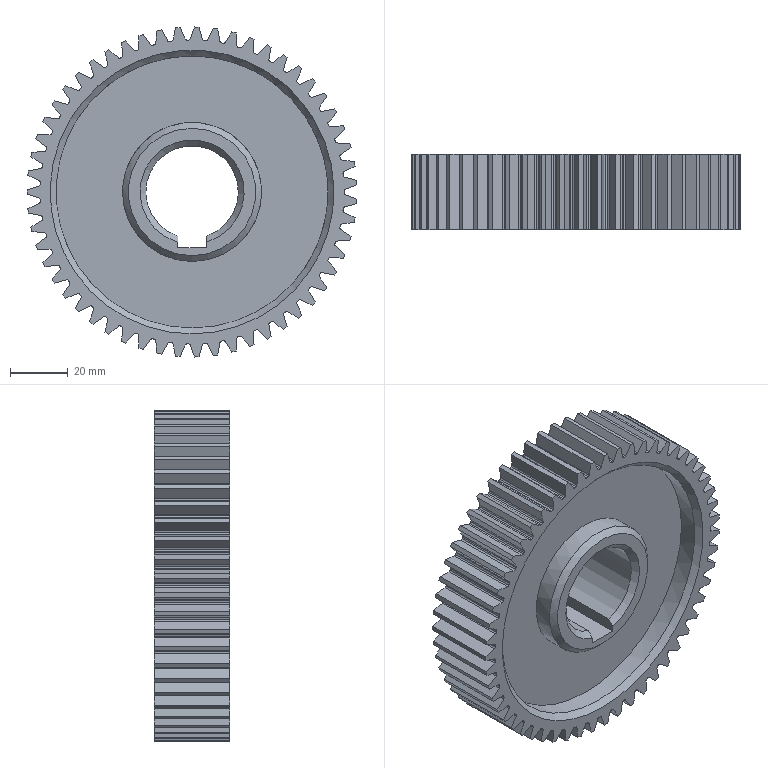Part | NX | features BREP 55, META 55, DATUM_CSYS 4, EXTRUDE 3, SKETCH 3, EXTRACT_DATUM_AXIS 2, EXTRACT_DATUM_PLANE 2, EXTRACT_STRING 2, CHAMFER 1, CYLINDER 1, FSET 1, Instance Feature 1, Mirror Feature 1 | 1 solid | 350 faces | box 113.946 x 26 x 113.987 mm | volume 134630 mm3 | spline 275 | cylinder 60 | plane 9 | cone 6 | commonest cylinder face diameters 105 x55 48 x2 94 x2 32 x1